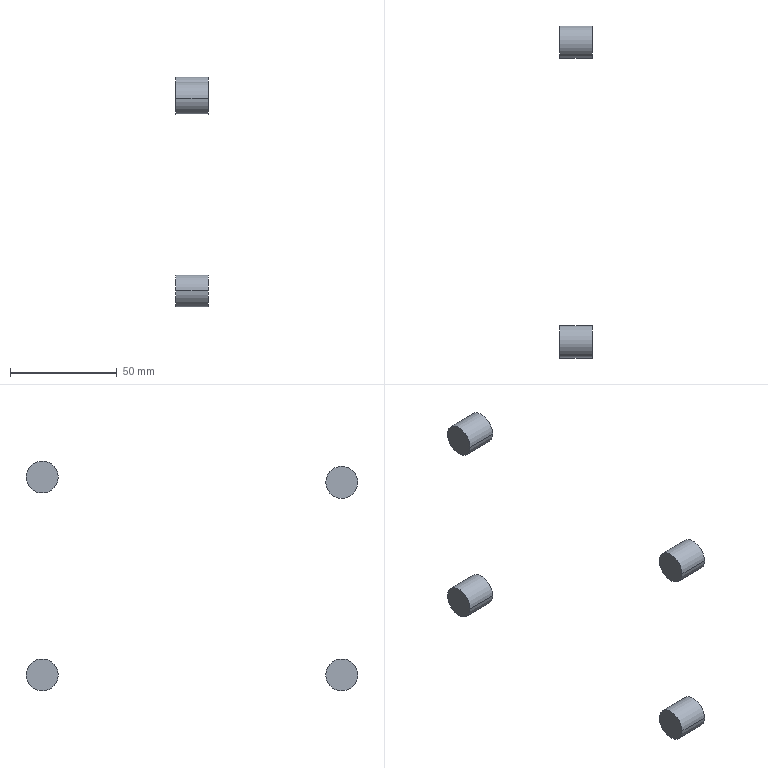Part | STEP file | PN_0011 | 4 solids | 16 faces | box 15 x 155 x 107.5 mm | volume 10603 mm3 | plane 8 | cylinder 8 | commonest cylinder face diameters 15 x8
STEP:
#1=CARTESIAN_POINT('',(0.,0.,0.));
#2=DIRECTION('',(0.,0.,1.));
#3=DIRECTION('',(1.,0.,0.));
#4=AXIS2_PLACEMENT_3D('',#1,#2,#3);
#5=CARTESIAN_POINT('',(15.,77.5,-43.));
#6=VERTEX_POINT('',#5);
#7=CARTESIAN_POINT('',(15.,62.5,-43.));
#8=VERTEX_POINT('',#7);
#9=CARTESIAN_POINT('',(15.,70.,-43.));
#10=DIRECTION('',(1.,0.,0.));
#11=DIRECTION('',(0.,1.,0.));
#12=AXIS2_PLACEMENT_3D('',#9,#10,#11);
#13=CIRCLE('',#12,7.5);
#14=CARTESIAN_POINT('',(15.,0.,0.));
#15=DIRECTION('',(1.,0.,0.));
#16=DIRECTION('',(0.,1.,0.));
#17=AXIS2_PLACEMENT_3D('',#14,#15,#16);
#18=PLANE('',#17);
#19=CARTESIAN_POINT('',(70.,-43.));
#20=DIRECTION('',(1.,0.));
#21=AXIS2_PLACEMENT_2D('',#19,#20);
#22=CIRCLE('',#21,7.5);
#23=(GEOMETRIC_REPRESENTATION_CONTEXT(2)PARAMETRIC_REPRESENTATION_CONTEXT()REPRESENTATION_CONTEXT('',''));
#24=DEFINITIONAL_REPRESENTATION('',(#22),#23);
#25=PCURVE('',#18,#24);
#26=CARTESIAN_POINT('',(15.,70.,-43.));
#27=DIRECTION('',(1.,0.,0.));
#28=DIRECTION('',(0.,1.,0.));
#29=AXIS2_PLACEMENT_3D('',#26,#27,#28);
#30=CYLINDRICAL_SURFACE('',#29,7.5);
#31=CARTESIAN_POINT('',(0.,0.));
#32=DIRECTION('',(1.,0.));
#33=VECTOR('',#32,1.);
#34=LINE('',#31,#33);
#35=(GEOMETRIC_REPRESENTATION_CONTEXT(2)PARAMETRIC_REPRESENTATION_CONTEXT()REPRESENTATION_CONTEXT('',''));
#36=DEFINITIONAL_REPRESENTATION('',(#34),#35);
#37=PCURVE('',#30,#36);
#38=SURFACE_CURVE('',#13,(#25,#37),.PCURVE_S1.);
#39=EDGE_CURVE('',#6,#8,#38,.T.);
#40=ORIENTED_EDGE('',*,*,#39,.T.);
#41=CARTESIAN_POINT('',(15.,70.,-43.));
#42=DIRECTION('',(1.,0.,0.));
#43=DIRECTION('',(0.,-1.,0.));
#44=AXIS2_PLACEMENT_3D('',#41,#42,#43);
#45=CIRCLE('',#44,7.5);
#46=CARTESIAN_POINT('',(70.,-43.));
#47=DIRECTION('',(-1.,0.));
#48=AXIS2_PLACEMENT_2D('',#46,#47);
#49=CIRCLE('',#48,7.5);
#50=(GEOMETRIC_REPRESENTATION_CONTEXT(2)PARAMETRIC_REPRESENTATION_CONTEXT()REPRESENTATION_CONTEXT('',''));
#51=DEFINITIONAL_REPRESENTATION('',(#49),#50);
#52=PCURVE('',#18,#51);
#53=CARTESIAN_POINT('',(15.,70.,-43.));
#54=DIRECTION('',(1.,0.,0.));
#55=DIRECTION('',(0.,1.,0.));
#56=AXIS2_PLACEMENT_3D('',#53,#54,#55);
#57=CYLINDRICAL_SURFACE('',#56,7.5);
#58=CARTESIAN_POINT('',(3.142,0.));
#59=DIRECTION('',(1.,0.));
#60=VECTOR('',#59,1.);
#61=LINE('',#58,#60);
#62=(GEOMETRIC_REPRESENTATION_CONTEXT(2)PARAMETRIC_REPRESENTATION_CONTEXT()REPRESENTATION_CONTEXT('',''));
#63=DEFINITIONAL_REPRESENTATION('',(#61),#62);
#64=PCURVE('',#57,#63);
#65=SURFACE_CURVE('',#45,(#52,#64),.PCURVE_S1.);
#66=EDGE_CURVE('',#8,#6,#65,.T.);
#67=ORIENTED_EDGE('',*,*,#66,.T.);
#68=EDGE_LOOP('',(#40,#67));
#69=FACE_BOUND('',#68,.F.);
#70=ADVANCED_FACE('',(#69),#18,.F.);
#71=CARTESIAN_POINT('',(30.,62.5,-43.));
#72=VERTEX_POINT('',#71);
#73=CARTESIAN_POINT('',(15.,62.5,-43.));
#74=DIRECTION('',(1.,0.,0.));
#75=VECTOR('',#74,1.);
#76=LINE('',#73,#75);
#77=CARTESIAN_POINT('',(3.142,0.));
#78=DIRECTION('',(0.,1.));
#79=VECTOR('',#78,1.);
#80=LINE('',#77,#79);
#81=(GEOMETRIC_REPRESENTATION_CONTEXT(2)PARAMETRIC_REPRESENTATION_CONTEXT()REPRESENTATION_CONTEXT('',''));
#82=DEFINITIONAL_REPRESENTATION('',(#80),#81);
#83=PCURVE('',#30,#82);
#84=CARTESIAN_POINT('',(3.142,0.));
#85=DIRECTION('',(0.,1.));
#86=VECTOR('',#85,1.);
#87=LINE('',#84,#86);
#88=(GEOMETRIC_REPRESENTATION_CONTEXT(2)PARAMETRIC_REPRESENTATION_CONTEXT()REPRESENTATION_CONTEXT('',''));
#89=DEFINITIONAL_REPRESENTATION('',(#87),#88);
#90=PCURVE('',#57,#89);
#91=SURFACE_CURVE('',#76,(#83,#90),.PCURVE_S1.);
#92=EDGE_CURVE('',#8,#72,#91,.T.);
#93=ORIENTED_EDGE('',*,*,#92,.T.);
#94=CARTESIAN_POINT('',(30.,77.5,-43.));
#95=VERTEX_POINT('',#94);
#96=CARTESIAN_POINT('',(30.,70.,-43.));
#97=DIRECTION('',(1.,0.,0.));
#98=DIRECTION('',(0.,1.,0.));
#99=AXIS2_PLACEMENT_3D('',#96,#97,#98);
#100=CIRCLE('',#99,7.5);
#101=CARTESIAN_POINT('',(0.,15.));
#102=DIRECTION('',(1.,0.));
#103=VECTOR('',#102,1.);
#104=LINE('',#101,#103);
#105=(GEOMETRIC_REPRESENTATION_CONTEXT(2)PARAMETRIC_REPRESENTATION_CONTEXT()REPRESENTATION_CONTEXT('',''));
#106=DEFINITIONAL_REPRESENTATION('',(#104),#105);
#107=PCURVE('',#30,#106);
#108=CARTESIAN_POINT('',(30.,0.,0.));
#109=DIRECTION('',(1.,0.,0.));
#110=DIRECTION('',(0.,1.,0.));
#111=AXIS2_PLACEMENT_3D('',#108,#109,#110);
#112=PLANE('',#111);
#113=CARTESIAN_POINT('',(70.,-43.));
#114=DIRECTION('',(1.,0.));
#115=AXIS2_PLACEMENT_2D('',#113,#114);
#116=CIRCLE('',#115,7.5);
#117=(GEOMETRIC_REPRESENTATION_CONTEXT(2)PARAMETRIC_REPRESENTATION_CONTEXT()REPRESENTATION_CONTEXT('',''));
#118=DEFINITIONAL_REPRESENTATION('',(#116),#117);
#119=PCURVE('',#112,#118);
#120=SURFACE_CURVE('',#100,(#107,#119),.PCURVE_S1.);
#121=EDGE_CURVE('',#95,#72,#120,.T.);
#122=ORIENTED_EDGE('',*,*,#121,.F.);
#123=CARTESIAN_POINT('',(15.,77.5,-43.));
#124=DIRECTION('',(1.,0.,0.));
#125=VECTOR('',#124,1.);
#126=LINE('',#123,#125);
#127=CARTESIAN_POINT('',(0.,0.));
#128=DIRECTION('',(0.,1.));
#129=VECTOR('',#128,1.);
#130=LINE('',#127,#129);
#131=(GEOMETRIC_REPRESENTATION_CONTEXT(2)PARAMETRIC_REPRESENTATION_CONTEXT()REPRESENTATION_CONTEXT('',''));
#132=DEFINITIONAL_REPRESENTATION('',(#130),#131);
#133=PCURVE('',#30,#132);
#134=CARTESIAN_POINT('',(6.283,0.));
#135=DIRECTION('',(0.,1.));
#136=VECTOR('',#135,1.);
#137=LINE('',#134,#136);
#138=(GEOMETRIC_REPRESENTATION_CONTEXT(2)PARAMETRIC_REPRESENTATION_CONTEXT()REPRESENTATION_CONTEXT('',''));
#139=DEFINITIONAL_REPRESENTATION('',(#137),#138);
#140=PCURVE('',#57,#139);
#141=SURFACE_CURVE('',#126,(#133,#140),.PCURVE_S1.);
#142=EDGE_CURVE('',#6,#95,#141,.T.);
#143=ORIENTED_EDGE('',*,*,#142,.F.);
#144=ORIENTED_EDGE('',*,*,#39,.T.);
#145=EDGE_LOOP('',(#93,#122,#143,#144));
#146=FACE_BOUND('',#145,.T.);
#147=ADVANCED_FACE('',(#146),#30,.T.);
#148=ORIENTED_EDGE('',*,*,#142,.T.);
#149=CARTESIAN_POINT('',(30.,70.,-43.));
#150=DIRECTION('',(1.,0.,0.));
#151=DIRECTION('',(0.,-1.,0.));
#152=AXIS2_PLACEMENT_3D('',#149,#150,#151);
#153=CIRCLE('',#152,7.5);
#154=CARTESIAN_POINT('',(3.142,15.));
#155=DIRECTION('',(1.,0.));
#156=VECTOR('',#155,1.);
#157=LINE('',#154,#156);
#158=(GEOMETRIC_REPRESENTATION_CONTEXT(2)PARAMETRIC_REPRESENTATION_CONTEXT()REPRESENTATION_CONTEXT('',''));
#159=DEFINITIONAL_REPRESENTATION('',(#157),#158);
#160=PCURVE('',#57,#159);
#161=CARTESIAN_POINT('',(70.,-43.));
#162=DIRECTION('',(-1.,0.));
#163=AXIS2_PLACEMENT_2D('',#161,#162);
#164=CIRCLE('',#163,7.5);
#165=(GEOMETRIC_REPRESENTATION_CONTEXT(2)PARAMETRIC_REPRESENTATION_CONTEXT()REPRESENTATION_CONTEXT('',''));
#166=DEFINITIONAL_REPRESENTATION('',(#164),#165);
#167=PCURVE('',#112,#166);
#168=SURFACE_CURVE('',#153,(#160,#167),.PCURVE_S1.);
#169=EDGE_CURVE('',#72,#95,#168,.T.);
#170=ORIENTED_EDGE('',*,*,#169,.F.);
#171=ORIENTED_EDGE('',*,*,#92,.F.);
#172=ORIENTED_EDGE('',*,*,#66,.T.);
#173=EDGE_LOOP('',(#148,#170,#171,#172));
#174=FACE_BOUND('',#173,.T.);
#175=ADVANCED_FACE('',(#174),#57,.T.);
#176=ORIENTED_EDGE('',*,*,#121,.F.);
#177=ORIENTED_EDGE('',*,*,#169,.F.);
#178=EDGE_LOOP('',(#176,#177));
#179=FACE_BOUND('',#178,.F.);
#180=ADVANCED_FACE('',(#179),#112,.T.);
#181=CLOSED_SHELL('',(#70,#147,#175,#180));
#182=MANIFOLD_SOLID_BREP('',#181);
#183=CARTESIAN_POINT('',(15.,-62.5,-43.));
#184=VERTEX_POINT('',#183);
#185=CARTESIAN_POINT('',(15.,-77.5,-43.));
#186=VERTEX_POINT('',#185);
#187=CARTESIAN_POINT('',(15.,-70.,-43.));
#188=DIRECTION('',(1.,0.,0.));
#189=DIRECTION('',(0.,1.,0.));
#190=AXIS2_PLACEMENT_3D('',#187,#188,#189);
#191=CIRCLE('',#190,7.5);
#192=CARTESIAN_POINT('',(15.,0.,0.));
#193=DIRECTION('',(1.,0.,0.));
#194=DIRECTION('',(0.,1.,0.));
#195=AXIS2_PLACEMENT_3D('',#192,#193,#194);
#196=PLANE('',#195);
#197=CARTESIAN_POINT('',(-70.,-43.));
#198=DIRECTION('',(1.,0.));
#199=AXIS2_PLACEMENT_2D('',#197,#198);
#200=CIRCLE('',#199,7.5);
#201=(GEOMETRIC_REPRESENTATION_CONTEXT(2)PARAMETRIC_REPRESENTATION_CONTEXT()REPRESENTATION_CONTEXT('',''));
#202=DEFINITIONAL_REPRESENTATION('',(#200),#201);
#203=PCURVE('',#196,#202);
#204=CARTESIAN_POINT('',(15.,-70.,-43.));
#205=DIRECTION('',(1.,0.,0.));
#206=DIRECTION('',(0.,1.,0.));
#207=AXIS2_PLACEMENT_3D('',#204,#205,#206);
#208=CYLINDRICAL_SURFACE('',#207,7.5);
#209=CARTESIAN_POINT('',(0.,0.));
#210=DIRECTION('',(1.,0.));
#211=VECTOR('',#210,1.);
#212=LINE('',#209,#211);
#213=(GEOMETRIC_REPRESENTATION_CONTEXT(2)PARAMETRIC_REPRESENTATION_CONTEXT()REPRESENTATION_CONTEXT('',''));
#214=DEFINITIONAL_REPRESENTATION('',(#212),#213);
#215=PCURVE('',#208,#214);
#216=SURFACE_CURVE('',#191,(#203,#215),.PCURVE_S1.);
#217=EDGE_CURVE('',#184,#186,#216,.T.);
#218=ORIENTED_EDGE('',*,*,#217,.T.);
#219=CARTESIAN_POINT('',(15.,-70.,-43.));
#220=DIRECTION('',(1.,0.,0.));
#221=DIRECTION('',(0.,-1.,0.));
#222=AXIS2_PLACEMENT_3D('',#219,#220,#221);
#223=CIRCLE('',#222,7.5);
#224=CARTESIAN_POINT('',(-70.,-43.));
#225=DIRECTION('',(-1.,0.));
#226=AXIS2_PLACEMENT_2D('',#224,#225);
#227=CIRCLE('',#226,7.5);
#228=(GEOMETRIC_REPRESENTATION_CONTEXT(2)PARAMETRIC_REPRESENTATION_CONTEXT()REPRESENTATION_CONTEXT('',''));
#229=DEFINITIONAL_REPRESENTATION('',(#227),#228);
#230=PCURVE('',#196,#229);
#231=CARTESIAN_POINT('',(15.,-70.,-43.));
#232=DIRECTION('',(1.,0.,0.));
#233=DIRECTION('',(0.,1.,0.));
#234=AXIS2_PLACEMENT_3D('',#231,#232,#233);
#235=CYLINDRICAL_SURFACE('',#234,7.5);
#236=CARTESIAN_POINT('',(3.142,0.));
#237=DIRECTION('',(1.,0.));
#238=VECTOR('',#237,1.);
#239=LINE('',#236,#238);
#240=(GEOMETRIC_REPRESENTATION_CONTEXT(2)PARAMETRIC_REPRESENTATION_CONTEXT()REPRESENTATION_CONTEXT('',''));
#241=DEFINITIONAL_REPRESENTATION('',(#239),#240);
#242=PCURVE('',#235,#241);
#243=SURFACE_CURVE('',#223,(#230,#242),.PCURVE_S1.);
#244=EDGE_CURVE('',#186,#184,#243,.T.);
#245=ORIENTED_EDGE('',*,*,#244,.T.);
#246=EDGE_LOOP('',(#218,#245));
#247=FACE_BOUND('',#246,.F.);
#248=ADVANCED_FACE('',(#247),#196,.F.);
#249=CARTESIAN_POINT('',(30.,-77.5,-43.));
#250=VERTEX_POINT('',#249);
#251=CARTESIAN_POINT('',(15.,-77.5,-43.));
#252=DIRECTION('',(1.,0.,0.));
#253=VECTOR('',#252,1.);
#254=LINE('',#251,#253);
#255=CARTESIAN_POINT('',(3.142,0.));
#256=DIRECTION('',(0.,1.));
#257=VECTOR('',#256,1.);
#258=LINE('',#255,#257);
#259=(GEOMETRIC_REPRESENTATION_CONTEXT(2)PARAMETRIC_REPRESENTATION_CONTEXT()REPRESENTATION_CONTEXT('',''));
#260=DEFINITIONAL_REPRESENTATION('',(#258),#259);
#261=PCURVE('',#208,#260);
#262=CARTESIAN_POINT('',(3.142,0.));
#263=DIRECTION('',(0.,1.));
#264=VECTOR('',#263,1.);
#265=LINE('',#262,#264);
#266=(GEOMETRIC_REPRESENTATION_CONTEXT(2)PARAMETRIC_REPRESENTATION_CONTEXT()REPRESENTATION_CONTEXT('',''));
#267=DEFINITIONAL_REPRESENTATION('',(#265),#266);
#268=PCURVE('',#235,#267);
#269=SURFACE_CURVE('',#254,(#261,#268),.PCURVE_S1.);
#270=EDGE_CURVE('',#186,#250,#269,.T.);
#271=ORIENTED_EDGE('',*,*,#270,.T.);
#272=CARTESIAN_POINT('',(30.,-62.5,-43.));
#273=VERTEX_POINT('',#272);
#274=CARTESIAN_POINT('',(30.,-70.,-43.));
#275=DIRECTION('',(1.,0.,0.));
#276=DIRECTION('',(0.,1.,0.));
#277=AXIS2_PLACEMENT_3D('',#274,#275,#276);
#278=CIRCLE('',#277,7.5);
#279=CARTESIAN_POINT('',(0.,15.));
#280=DIRECTION('',(1.,0.));
#281=VECTOR('',#280,1.);
#282=LINE('',#279,#281);
#283=(GEOMETRIC_REPRESENTATION_CONTEXT(2)PARAMETRIC_REPRESENTATION_CONTEXT()REPRESENTATION_CONTEXT('',''));
#284=DEFINITIONAL_REPRESENTATION('',(#282),#283);
#285=PCURVE('',#208,#284);
#286=CARTESIAN_POINT('',(30.,0.,0.));
#287=DIRECTION('',(1.,0.,0.));
#288=DIRECTION('',(0.,1.,0.));
#289=AXIS2_PLACEMENT_3D('',#286,#287,#288);
#290=PLANE('',#289);
#291=CARTESIAN_POINT('',(-70.,-43.));
#292=DIRECTION('',(1.,0.));
#293=AXIS2_PLACEMENT_2D('',#291,#292);
#294=CIRCLE('',#293,7.5);
#295=(GEOMETRIC_REPRESENTATION_CONTEXT(2)PARAMETRIC_REPRESENTATION_CONTEXT()REPRESENTATION_CONTEXT('',''));
#296=DEFINITIONAL_REPRESENTATION('',(#294),#295);
#297=PCURVE('',#290,#296);
#298=SURFACE_CURVE('',#278,(#285,#297),.PCURVE_S1.);
#299=EDGE_CURVE('',#273,#250,#298,.T.);
#300=ORIENTED_EDGE('',*,*,#299,.F.);
#301=CARTESIAN_POINT('',(15.,-62.5,-43.));
#302=DIRECTION('',(1.,0.,0.));
#303=VECTOR('',#302,1.);
#304=LINE('',#301,#303);
#305=CARTESIAN_POINT('',(0.,0.));
#306=DIRECTION('',(0.,1.));
#307=VECTOR('',#306,1.);
#308=LINE('',#305,#307);
#309=(GEOMETRIC_REPRESENTATION_CONTEXT(2)PARAMETRIC_REPRESENTATION_CONTEXT()REPRESENTATION_CONTEXT('',''));
#310=DEFINITIONAL_REPRESENTATION('',(#308),#309);
#311=PCURVE('',#208,#310);
#312=CARTESIAN_POINT('',(6.283,0.));
#313=DIRECTION('',(0.,1.));
#314=VECTOR('',#313,1.);
#315=LINE('',#312,#314);
#316=(GEOMETRIC_REPRESENTATION_CONTEXT(2)PARAMETRIC_REPRESENTATION_CONTEXT()REPRESENTATION_CONTEXT('',''));
#317=DEFINITIONAL_REPRESENTATION('',(#315),#316);
#318=PCURVE('',#235,#317);
#319=SURFACE_CURVE('',#304,(#311,#318),.PCURVE_S1.);
#320=EDGE_CURVE('',#184,#273,#319,.T.);
#321=ORIENTED_EDGE('',*,*,#320,.F.);
#322=ORIENTED_EDGE('',*,*,#217,.T.);
#323=EDGE_LOOP('',(#271,#300,#321,#322));
#324=FACE_BOUND('',#323,.T.);
#325=ADVANCED_FACE('',(#324),#208,.T.);
#326=ORIENTED_EDGE('',*,*,#320,.T.);
#327=CARTESIAN_POINT('',(30.,-70.,-43.));
#328=DIRECTION('',(1.,0.,0.));
#329=DIRECTION('',(0.,-1.,0.));
#330=AXIS2_PLACEMENT_3D('',#327,#328,#329);
#331=CIRCLE('',#330,7.5);
#332=CARTESIAN_POINT('',(3.142,15.));
#333=DIRECTION('',(1.,0.));
#334=VECTOR('',#333,1.);
#335=LINE('',#332,#334);
#336=(GEOMETRIC_REPRESENTATION_CONTEXT(2)PARAMETRIC_REPRESENTATION_CONTEXT()REPRESENTATION_CONTEXT('',''));
#337=DEFINITIONAL_REPRESENTATION('',(#335),#336);
#338=PCURVE('',#235,#337);
#339=CARTESIAN_POINT('',(-70.,-43.));
#340=DIRECTION('',(-1.,0.));
#341=AXIS2_PLACEMENT_2D('',#339,#340);
#342=CIRCLE('',#341,7.5);
#343=(GEOMETRIC_REPRESENTATION_CONTEXT(2)PARAMETRIC_REPRESENTATION_CONTEXT()REPRESENTATION_CONTEXT('',''));
#344=DEFINITIONAL_REPRESENTATION('',(#342),#343);
#345=PCURVE('',#290,#344);
#346=SURFACE_CURVE('',#331,(#338,#345),.PCURVE_S1.);
#347=EDGE_CURVE('',#250,#273,#346,.T.);
#348=ORIENTED_EDGE('',*,*,#347,.F.);
#349=ORIENTED_EDGE('',*,*,#270,.F.);
#350=ORIENTED_EDGE('',*,*,#244,.T.);
#351=EDGE_LOOP('',(#326,#348,#349,#350));
#352=FACE_BOUND('',#351,.T.);
#353=ADVANCED_FACE('',(#352),#235,.T.);
#354=ORIENTED_EDGE('',*,*,#299,.F.);
#355=ORIENTED_EDGE('',*,*,#347,.F.);
#356=EDGE_LOOP('',(#354,#355));
#357=FACE_BOUND('',#356,.F.);
#358=ADVANCED_FACE('',(#357),#290,.T.);
#359=CLOSED_SHELL('',(#248,#325,#353,#358));
#360=MANIFOLD_SOLID_BREP('',#359);
#361=CARTESIAN_POINT('',(15.,-62.5,47.));
#362=VERTEX_POINT('',#361);
#363=CARTESIAN_POINT('',(15.,-77.5,47.));
#364=VERTEX_POINT('',#363);
#365=CARTESIAN_POINT('',(15.,-70.,47.));
#366=DIRECTION('',(1.,0.,0.));
#367=DIRECTION('',(0.,1.,0.));
#368=AXIS2_PLACEMENT_3D('',#365,#366,#367);
#369=CIRCLE('',#368,7.5);
#370=CARTESIAN_POINT('',(15.,0.,0.));
#371=DIRECTION('',(1.,0.,0.));
#372=DIRECTION('',(0.,1.,0.));
#373=AXIS2_PLACEMENT_3D('',#370,#371,#372);
#374=PLANE('',#373);
#375=CARTESIAN_POINT('',(-70.,47.));
#376=DIRECTION('',(1.,0.));
#377=AXIS2_PLACEMENT_2D('',#375,#376);
#378=CIRCLE('',#377,7.5);
#379=(GEOMETRIC_REPRESENTATION_CONTEXT(2)PARAMETRIC_REPRESENTATION_CONTEXT()REPRESENTATION_CONTEXT('',''));
#380=DEFINITIONAL_REPRESENTATION('',(#378),#379);
#381=PCURVE('',#374,#380);
#382=CARTESIAN_POINT('',(15.,-70.,47.));
#383=DIRECTION('',(1.,0.,0.));
#384=DIRECTION('',(0.,1.,0.));
#385=AXIS2_PLACEMENT_3D('',#382,#383,#384);
#386=CYLINDRICAL_SURFACE('',#385,7.5);
#387=CARTESIAN_POINT('',(0.,0.));
#388=DIRECTION('',(1.,0.));
#389=VECTOR('',#388,1.);
#390=LINE('',#387,#389);
#391=(GEOMETRIC_REPRESENTATION_CONTEXT(2)PARAMETRIC_REPRESENTATION_CONTEXT()REPRESENTATION_CONTEXT('',''));
#392=DEFINITIONAL_REPRESENTATION('',(#390),#391);
#393=PCURVE('',#386,#392);
#394=SURFACE_CURVE('',#369,(#381,#393),.PCURVE_S1.);
#395=EDGE_CURVE('',#362,#364,#394,.T.);
#396=ORIENTED_EDGE('',*,*,#395,.T.);
#397=CARTESIAN_POINT('',(15.,-70.,47.));
#398=DIRECTION('',(1.,0.,0.));
#399=DIRECTION('',(0.,-1.,0.));
#400=AXIS2_PLACEMENT_3D('',#397,#398,#399);
#401=CIRCLE('',#400,7.5);
#402=CARTESIAN_POINT('',(-70.,47.));
#403=DIRECTION('',(-1.,0.));
#404=AXIS2_PLACEMENT_2D('',#402,#403);
#405=CIRCLE('',#404,7.5);
#406=(GEOMETRIC_REPRESENTATION_CONTEXT(2)PARAMETRIC_REPRESENTATION_CONTEXT()REPRESENTATION_CONTEXT('',''));
#407=DEFINITIONAL_REPRESENTATION('',(#405),#406);
#408=PCURVE('',#374,#407);
#409=CARTESIAN_POINT('',(15.,-70.,47.));
#410=DIRECTION('',(1.,0.,0.));
#411=DIRECTION('',(0.,1.,0.));
#412=AXIS2_PLACEMENT_3D('',#409,#410,#411);
#413=CYLINDRICAL_SURFACE('',#412,7.5);
#414=CARTESIAN_POINT('',(3.142,0.));
#415=DIRECTION('',(1.,0.));
#416=VECTOR('',#415,1.);
#417=LINE('',#414,#416);
#418=(GEOMETRIC_REPRESENTATION_CONTEXT(2)PARAMETRIC_REPRESENTATION_CONTEXT()REPRESENTATION_CONTEXT('',''));
#419=DEFINITIONAL_REPRESENTATION('',(#417),#418);
#420=PCURVE('',#413,#419);
#421=SURFACE_CURVE('',#401,(#408,#420),.PCURVE_S1.);
#422=EDGE_CURVE('',#364,#362,#421,.T.);
#423=ORIENTED_EDGE('',*,*,#422,.T.);
#424=EDGE_LOOP('',(#396,#423));
#425=FACE_BOUND('',#424,.F.);
#426=ADVANCED_FACE('',(#425),#374,.F.);
#427=CARTESIAN_POINT('',(30.,-77.5,47.));
#428=VERTEX_POINT('',#427);
#429=CARTESIAN_POINT('',(15.,-77.5,47.));
#430=DIRECTION('',(1.,0.,0.));
#431=VECTOR('',#430,1.);
#432=LINE('',#429,#431);
#433=CARTESIAN_POINT('',(3.142,0.));
#434=DIRECTION('',(0.,1.));
#435=VECTOR('',#434,1.);
#436=LINE('',#433,#435);
#437=(GEOMETRIC_REPRESENTATION_CONTEXT(2)PARAMETRIC_REPRESENTATION_CONTEXT()REPRESENTATION_CONTEXT('',''));
#438=DEFINITIONAL_REPRESENTATION('',(#436),#437);
#439=PCURVE('',#386,#438);
#440=CARTESIAN_POINT('',(3.142,0.));
#441=DIRECTION('',(0.,1.));
#442=VECTOR('',#441,1.);
#443=LINE('',#440,#442);
#444=(GEOMETRIC_REPRESENTATION_CONTEXT(2)PARAMETRIC_REPRESENTATION_CONTEXT()REPRESENTATION_CONTEXT('',''));
#445=DEFINITIONAL_REPRESENTATION('',(#443),#444);
#446=PCURVE('',#413,#445);
#447=SURFACE_CURVE('',#432,(#439,#446),.PCURVE_S1.);
#448=EDGE_CURVE('',#364,#428,#447,.T.);
#449=ORIENTED_EDGE('',*,*,#448,.T.);
#450=CARTESIAN_POINT('',(30.,-62.5,47.));
#451=VERTEX_POINT('',#450);
#452=CARTESIAN_POINT('',(30.,-70.,47.));
#453=DIRECTION('',(1.,0.,0.));
#454=DIRECTION('',(0.,1.,0.));
#455=AXIS2_PLACEMENT_3D('',#452,#453,#454);
#456=CIRCLE('',#455,7.5);
#457=CARTESIAN_POINT('',(0.,15.));
#458=DIRECTION('',(1.,0.));
#459=VECTOR('',#458,1.);
#460=LINE('',#457,#459);
#461=(GEOMETRIC_REPRESENTATION_CONTEXT(2)PARAMETRIC_REPRESENTATION_CONTEXT()REPRESENTATION_CONTEXT('',''));
#462=DEFINITIONAL_REPRESENTATION('',(#460),#461);
#463=PCURVE('',#386,#462);
#464=CARTESIAN_POINT('',(30.,0.,0.));
#465=DIRECTION('',(1.,0.,0.));
#466=DIRECTION('',(0.,1.,0.));
#467=AXIS2_PLACEMENT_3D('',#464,#465,#466);
#468=PLANE('',#467);
#469=CARTESIAN_POINT('',(-70.,47.));
#470=DIRECTION('',(1.,0.));
#471=AXIS2_PLACEMENT_2D('',#469,#470);
#472=CIRCLE('',#471,7.5);
#473=(GEOMETRIC_REPRESENTATION_CONTEXT(2)PARAMETRIC_REPRESENTATION_CONTEXT()REPRESENTATION_CONTEXT('',''));
#474=DEFINITIONAL_REPRESENTATION('',(#472),#473);
#475=PCURVE('',#468,#474);
#476=SURFACE_CURVE('',#456,(#463,#475),.PCURVE_S1.);
#477=EDGE_CURVE('',#451,#428,#476,.T.);
#478=ORIENTED_EDGE('',*,*,#477,.F.);
#479=CARTESIAN_POINT('',(15.,-62.5,47.));
#480=DIRECTION('',(1.,0.,0.));
#481=VECTOR('',#480,1.);
#482=LINE('',#479,#481);
#483=CARTESIAN_POINT('',(0.,0.));
#484=DIRECTION('',(0.,1.));
#485=VECTOR('',#484,1.);
#486=LINE('',#483,#485);
#487=(GEOMETRIC_REPRESENTATION_CONTEXT(2)PARAMETRIC_REPRESENTATION_CONTEXT()REPRESENTATION_CONTEXT('',''));
#488=DEFINITIONAL_REPRESENTATION('',(#486),#487);
#489=PCURVE('',#386,#488);
#490=CARTESIAN_POINT('',(6.283,0.));
#491=DIRECTION('',(0.,1.));
#492=VECTOR('',#491,1.);
#493=LINE('',#490,#492);
#494=(GEOMETRIC_REPRESENTATION_CONTEXT(2)PARAMETRIC_REPRESENTATION_CONTEXT()REPRESENTATION_CONTEXT('',''));
#495=DEFINITIONAL_REPRESENTATION('',(#493),#494);
#496=PCURVE('',#413,#495);
#497=SURFACE_CURVE('',#482,(#489,#496),.PCURVE_S1.);
#498=EDGE_CURVE('',#362,#451,#497,.T.);
#499=ORIENTED_EDGE('',*,*,#498,.F.);
#500=ORIENTED_EDGE('',*,*,#395,.T.);
#501=EDGE_LOOP('',(#449,#478,#499,#500));
#502=FACE_BOUND('',#501,.T.);
#503=ADVANCED_FACE('',(#502),#386,.T.);
#504=ORIENTED_EDGE('',*,*,#498,.T.);
#505=CARTESIAN_POINT('',(30.,-70.,47.));
#506=DIRECTION('',(1.,0.,0.));
#507=DIRECTION('',(0.,-1.,0.));
#508=AXIS2_PLACEMENT_3D('',#505,#506,#507);
#509=CIRCLE('',#508,7.5);
#510=CARTESIAN_POINT('',(3.142,15.));
#511=DIRECTION('',(1.,0.));
#512=VECTOR('',#511,1.);
#513=LINE('',#510,#512);
#514=(GEOMETRIC_REPRESENTATION_CONTEXT(2)PARAMETRIC_REPRESENTATION_CONTEXT()REPRESENTATION_CONTEXT('',''));
#515=DEFINITIONAL_REPRESENTATION('',(#513),#514);
#516=PCURVE('',#413,#515);
#517=CARTESIAN_POINT('',(-70.,47.));
#518=DIRECTION('',(-1.,0.));
#519=AXIS2_PLACEMENT_2D('',#517,#518);
#520=CIRCLE('',#519,7.5);
#521=(GEOMETRIC_REPRESENTATION_CONTEXT(2)PARAMETRIC_REPRESENTATION_CONTEXT()REPRESENTATION_CONTEXT('',''));
#522=DEFINITIONAL_REPRESENTATION('',(#520),#521);
#523=PCURVE('',#468,#522);
#524=SURFACE_CURVE('',#509,(#516,#523),.PCURVE_S1.);
#525=EDGE_CURVE('',#428,#451,#524,.T.);
#526=ORIENTED_EDGE('',*,*,#525,.F.);
#527=ORIENTED_EDGE('',*,*,#448,.F.);
#528=ORIENTED_EDGE('',*,*,#422,.T.);
#529=EDGE_LOOP('',(#504,#526,#527,#528));
#530=FACE_BOUND('',#529,.T.);
#531=ADVANCED_FACE('',(#530),#413,.T.);
#532=ORIENTED_EDGE('',*,*,#477,.F.);
#533=ORIENTED_EDGE('',*,*,#525,.F.);
#534=EDGE_LOOP('',(#532,#533));
#535=FACE_BOUND('',#534,.F.);
#536=ADVANCED_FACE('',(#535),#468,.T.);
#537=CLOSED_SHELL('',(#426,#503,#531,#536));
#538=MANIFOLD_SOLID_BREP('',#537);
#539=CARTESIAN_POINT('',(15.,77.5,49.5));
#540=VERTEX_POINT('',#539);
#541=CARTESIAN_POINT('',(15.,62.5,49.5));
#542=VERTEX_POINT('',#541);
#543=CARTESIAN_POINT('',(15.,70.,49.5));
#544=DIRECTION('',(1.,0.,0.));
#545=DIRECTION('',(0.,1.,0.));
#546=AXIS2_PLACEMENT_3D('',#543,#544,#545);
#547=CIRCLE('',#546,7.5);
#548=CARTESIAN_POINT('',(15.,0.,0.));
#549=DIRECTION('',(1.,0.,0.));
#550=DIRECTION('',(0.,1.,0.));
#551=AXIS2_PLACEMENT_3D('',#548,#549,#550);
#552=PLANE('',#551);
#553=CARTESIAN_POINT('',(70.,49.5));
#554=DIRECTION('',(1.,0.));
#555=AXIS2_PLACEMENT_2D('',#553,#554);
#556=CIRCLE('',#555,7.5);
#557=(GEOMETRIC_REPRESENTATION_CONTEXT(2)PARAMETRIC_REPRESENTATION_CONTEXT()REPRESENTATION_CONTEXT('',''));
#558=DEFINITIONAL_REPRESENTATION('',(#556),#557);
#559=PCURVE('',#552,#558);
#560=CARTESIAN_POINT('',(15.,70.,49.5));
#561=DIRECTION('',(1.,0.,0.));
#562=DIRECTION('',(0.,1.,0.));
#563=AXIS2_PLACEMENT_3D('',#560,#561,#562);
#564=CYLINDRICAL_SURFACE('',#563,7.5);
#565=CARTESIAN_POINT('',(0.,0.));
#566=DIRECTION('',(1.,0.));
#567=VECTOR('',#566,1.);
#568=LINE('',#565,#567);
#569=(GEOMETRIC_REPRESENTATION_CONTEXT(2)PARAMETRIC_REPRESENTATION_CONTEXT()REPRESENTATION_CONTEXT('',''));
#570=DEFINITIONAL_REPRESENTATION('',(#568),#569);
#571=PCURVE('',#564,#570);
#572=SURFACE_CURVE('',#547,(#559,#571),.PCURVE_S1.);
#573=EDGE_CURVE('',#540,#542,#572,.T.);
#574=ORIENTED_EDGE('',*,*,#573,.T.);
#575=CARTESIAN_POINT('',(15.,70.,49.5));
#576=DIRECTION('',(1.,0.,0.));
#577=DIRECTION('',(0.,-1.,0.));
#578=AXIS2_PLACEMENT_3D('',#575,#576,#577);
#579=CIRCLE('',#578,7.5);
#580=CARTESIAN_POINT('',(70.,49.5));
#581=DIRECTION('',(-1.,0.));
#582=AXIS2_PLACEMENT_2D('',#580,#581);
#583=CIRCLE('',#582,7.5);
#584=(GEOMETRIC_REPRESENTATION_CONTEXT(2)PARAMETRIC_REPRESENTATION_CONTEXT()REPRESENTATION_CONTEXT('',''));
#585=DEFINITIONAL_REPRESENTATION('',(#583),#584);
#586=PCURVE('',#552,#585);
#587=CARTESIAN_POINT('',(15.,70.,49.5));
#588=DIRECTION('',(1.,0.,0.));
#589=DIRECTION('',(0.,1.,0.));
#590=AXIS2_PLACEMENT_3D('',#587,#588,#589);
#591=CYLINDRICAL_SURFACE('',#590,7.5);
#592=CARTESIAN_POINT('',(3.142,0.));
#593=DIRECTION('',(1.,0.));
#594=VECTOR('',#593,1.);
#595=LINE('',#592,#594);
#596=(GEOMETRIC_REPRESENTATION_CONTEXT(2)PARAMETRIC_REPRESENTATION_CONTEXT()REPRESENTATION_CONTEXT('',''));
#597=DEFINITIONAL_REPRESENTATION('',(#595),#596);
#598=PCURVE('',#591,#597);
#599=SURFACE_CURVE('',#579,(#586,#598),.PCURVE_S1.);
#600=EDGE_CURVE('',#542,#540,#599,.T.);
#601=ORIENTED_EDGE('',*,*,#600,.T.);
#602=EDGE_LOOP('',(#574,#601));
#603=FACE_BOUND('',#602,.F.);
#604=ADVANCED_FACE('',(#603),#552,.F.);
#605=CARTESIAN_POINT('',(30.,62.5,49.5));
#606=VERTEX_POINT('',#605);
#607=CARTESIAN_POINT('',(15.,62.5,49.5));
#608=DIRECTION('',(1.,0.,0.));
#609=VECTOR('',#608,1.);
#610=LINE('',#607,#609);
#611=CARTESIAN_POINT('',(3.142,0.));
#612=DIRECTION('',(0.,1.));
#613=VECTOR('',#612,1.);
#614=LINE('',#611,#613);
#615=(GEOMETRIC_REPRESENTATION_CONTEXT(2)PARAMETRIC_REPRESENTATION_CONTEXT()REPRESENTATION_CONTEXT('',''));
#616=DEFINITIONAL_REPRESENTATION('',(#614),#615);
#617=PCURVE('',#564,#616);
#618=CARTESIAN_POINT('',(3.142,0.));
#619=DIRECTION('',(0.,1.));
#620=VECTOR('',#619,1.);
#621=LINE('',#618,#620);
#622=(GEOMETRIC_REPRESENTATION_CONTEXT(2)PARAMETRIC_REPRESENTATION_CONTEXT()REPRESENTATION_CONTEXT('',''));
#623=DEFINITIONAL_REPRESENTATION('',(#621),#622);
#624=PCURVE('',#591,#623);
#625=SURFACE_CURVE('',#610,(#617,#624),.PCURVE_S1.);
#626=EDGE_CURVE('',#542,#606,#625,.T.);
#627=ORIENTED_EDGE('',*,*,#626,.T.);
#628=CARTESIAN_POINT('',(30.,77.5,49.5));
#629=VERTEX_POINT('',#628);
#630=CARTESIAN_POINT('',(30.,70.,49.5));
#631=DIRECTION('',(1.,0.,0.));
#632=DIRECTION('',(0.,1.,0.));
#633=AXIS2_PLACEMENT_3D('',#630,#631,#632);
#634=CIRCLE('',#633,7.5);
#635=CARTESIAN_POINT('',(0.,15.));
#636=DIRECTION('',(1.,0.));
#637=VECTOR('',#636,1.);
#638=LINE('',#635,#637);
#639=(GEOMETRIC_REPRESENTATION_CONTEXT(2)PARAMETRIC_REPRESENTATION_CONTEXT()REPRESENTATION_CONTEXT('',''));
#640=DEFINITIONAL_REPRESENTATION('',(#638),#639);
#641=PCURVE('',#564,#640);
#642=CARTESIAN_POINT('',(30.,0.,0.));
#643=DIRECTION('',(1.,0.,0.));
#644=DIRECTION('',(0.,1.,0.));
#645=AXIS2_PLACEMENT_3D('',#642,#643,#644);
#646=PLANE('',#645);
#647=CARTESIAN_POINT('',(70.,49.5));
#648=DIRECTION('',(1.,0.));
#649=AXIS2_PLACEMENT_2D('',#647,#648);
#650=CIRCLE('',#649,7.5);
#651=(GEOMETRIC_REPRESENTATION_CONTEXT(2)PARAMETRIC_REPRESENTATION_CONTEXT()REPRESENTATION_CONTEXT('',''));
#652=DEFINITIONAL_REPRESENTATION('',(#650),#651);
#653=PCURVE('',#646,#652);
#654=SURFACE_CURVE('',#634,(#641,#653),.PCURVE_S1.);
#655=EDGE_CURVE('',#629,#606,#654,.T.);
#656=ORIENTED_EDGE('',*,*,#655,.F.);
#657=CARTESIAN_POINT('',(15.,77.5,49.5));
#658=DIRECTION('',(1.,0.,0.));
#659=VECTOR('',#658,1.);
#660=LINE('',#657,#659);
#661=CARTESIAN_POINT('',(0.,0.));
#662=DIRECTION('',(0.,1.));
#663=VECTOR('',#662,1.);
#664=LINE('',#661,#663);
#665=(GEOMETRIC_REPRESENTATION_CONTEXT(2)PARAMETRIC_REPRESENTATION_CONTEXT()REPRESENTATION_CONTEXT('',''));
#666=DEFINITIONAL_REPRESENTATION('',(#664),#665);
#667=PCURVE('',#564,#666);
#668=CARTESIAN_POINT('',(6.283,0.));
#669=DIRECTION('',(0.,1.));
#670=VECTOR('',#669,1.);
#671=LINE('',#668,#670);
#672=(GEOMETRIC_REPRESENTATION_CONTEXT(2)PARAMETRIC_REPRESENTATION_CONTEXT()REPRESENTATION_CONTEXT('',''));
#673=DEFINITIONAL_REPRESENTATION('',(#671),#672);
#674=PCURVE('',#591,#673);
#675=SURFACE_CURVE('',#660,(#667,#674),.PCURVE_S1.);
#676=EDGE_CURVE('',#540,#629,#675,.T.);
#677=ORIENTED_EDGE('',*,*,#676,.F.);
#678=ORIENTED_EDGE('',*,*,#573,.T.);
#679=EDGE_LOOP('',(#627,#656,#677,#678));
#680=FACE_BOUND('',#679,.T.);
#681=ADVANCED_FACE('',(#680),#564,.T.);
#682=ORIENTED_EDGE('',*,*,#676,.T.);
#683=CARTESIAN_POINT('',(30.,70.,49.5));
#684=DIRECTION('',(1.,0.,0.));
#685=DIRECTION('',(0.,-1.,0.));
#686=AXIS2_PLACEMENT_3D('',#683,#684,#685);
#687=CIRCLE('',#686,7.5);
#688=CARTESIAN_POINT('',(3.142,15.));
#689=DIRECTION('',(1.,0.));
#690=VECTOR('',#689,1.);
#691=LINE('',#688,#690);
#692=(GEOMETRIC_REPRESENTATION_CONTEXT(2)PARAMETRIC_REPRESENTATION_CONTEXT()REPRESENTATION_CONTEXT('',''));
#693=DEFINITIONAL_REPRESENTATION('',(#691),#692);
#694=PCURVE('',#591,#693);
#695=CARTESIAN_POINT('',(70.,49.5));
#696=DIRECTION('',(-1.,0.));
#697=AXIS2_PLACEMENT_2D('',#695,#696);
#698=CIRCLE('',#697,7.5);
#699=(GEOMETRIC_REPRESENTATION_CONTEXT(2)PARAMETRIC_REPRESENTATION_CONTEXT()REPRESENTATION_CONTEXT('',''));
#700=DEFINITIONAL_REPRESENTATION('',(#698),#699);
#701=PCURVE('',#646,#700);
#702=SURFACE_CURVE('',#687,(#694,#701),.PCURVE_S1.);
#703=EDGE_CURVE('',#606,#629,#702,.T.);
#704=ORIENTED_EDGE('',*,*,#703,.F.);
#705=ORIENTED_EDGE('',*,*,#626,.F.);
#706=ORIENTED_EDGE('',*,*,#600,.T.);
#707=EDGE_LOOP('',(#682,#704,#705,#706));
#708=FACE_BOUND('',#707,.T.);
#709=ADVANCED_FACE('',(#708),#591,.T.);
#710=ORIENTED_EDGE('',*,*,#655,.F.);
#711=ORIENTED_EDGE('',*,*,#703,.F.);
#712=EDGE_LOOP('',(#710,#711));
#713=FACE_BOUND('',#712,.F.);
#714=ADVANCED_FACE('',(#713),#646,.T.);
#715=CLOSED_SHELL('',(#604,#681,#709,#714));
#716=MANIFOLD_SOLID_BREP('',#715);
#717=(LENGTH_UNIT()NAMED_UNIT(*)SI_UNIT(.MILLI.,.METRE.));
#718=UNCERTAINTY_MEASURE_WITH_UNIT(LENGTH_MEASURE(0.0000001),#717,'','');
#719=(NAMED_UNIT(*)PLANE_ANGLE_UNIT()SI_UNIT($,.RADIAN.));
#720=(NAMED_UNIT(*)SI_UNIT($,.STERADIAN.)SOLID_ANGLE_UNIT());
#721=(GEOMETRIC_REPRESENTATION_CONTEXT(3)GLOBAL_UNCERTAINTY_ASSIGNED_CONTEXT((#718))GLOBAL_UNIT_ASSIGNED_CONTEXT((#717,#719,#720))REPRESENTATION_CONTEXT('',''));
#722=SHAPE_REPRESENTATION('',(#4,#182,#360,#538,#716),#721);